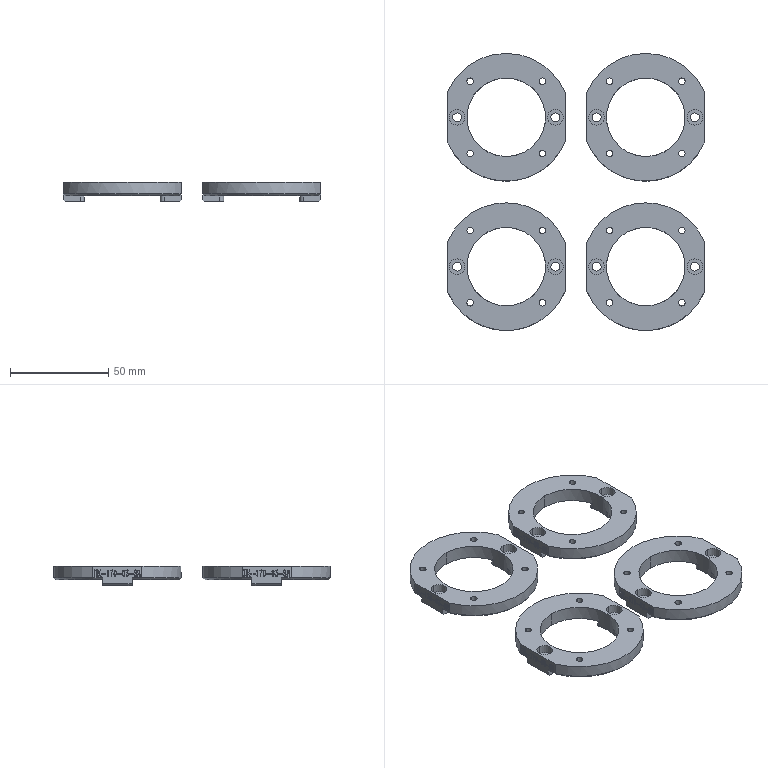NC program | NX | posted with a generic post | part box 131 x 141 x 10 mm
Whole program:
N10 G17 G21 G94 G90
(HOLE_MILLING_1 , TOOL : D6)
N12 T12 M6
N14 G54
N16 G17 G0 G90 X0. Y25. S9500 M3
N18 G43 Z30. H12
N20 Z0.5
N22 G94 G3 X0.5 Y25.5 R0.5 F1450.
N24 X0. Y26. R0.5
N26 X0. Y26. Z0. I0. J-1.
N28 X0. Y26. Z-0.5 I0. J-1.
N30 X0. Y26. Z-1. I0. J-1.
N32 X0. Y26. Z-1.5 I0. J-1.
N34 X0. Y26. Z-2. I0. J-1.
N36 X0. Y26. Z-2.5 I0. J-1.
N38 X0. Y26. Z-3. I0. J-1.
N40 X0. Y26. Z-3.5 I0. J-1.
N42 X0. Y26. Z-4. I0. J-1.
N44 X0.951 Y25.309 Z-4.4 R-1.
N46 X-0.309 Y25.951 R1.
N48 X0.951 Y25.309 R-1.
N50 X0.321 Y25.63 R0.5
N52 X0. Y25. R0.5
N54 G0 Z30.
N56 Y-25.
N58 Z0.5
N60 G3 X0.5 Y-24.5 R0.5
N62 X0. Y-24. R0.5
N64 X0. Y-24. Z0. I0. J-1.
N66 X0. Y-24. Z-0.5 I0. J-1.
N68 X0. Y-24. Z-1. I0. J-1.
N70 X0. Y-24. Z-1.5 I0. J-1.
N72 X0. Y-24. Z-2. I0. J-1.
N74 X0. Y-24. Z-2.5 I0. J-1.
N76 X0. Y-24. Z-3. I0. J-1.
N78 X0. Y-24. Z-3.5 I0. J-1.
N80 X0. Y-24. Z-4. I0. J-1.
N82 X0.951 Y-24.691 Z-4.4 R-1.
N84 X-0.309 Y-24.049 R1.
N86 X0.951 Y-24.691 R-1.
N88 X0.321 Y-24.37 R0.5
N90 X0. Y-25. R0.5
N92 G0 Z30.
N94 M5
(PLANAR_MILL_COPY_COPY_COPY_COPY_COPY_1 , TOOL : D6A45)
N96 T01 M6
N98 G54
N100 G17 G0 G90 X18.452 Y18.385 S9500 M3
N102 G43 Z30. H1
N104 Z0.
N106 G94 G1 Z-1.5 F1250.
N108 G3 X18.385 Y18.635 R0.5
N110 X18.135 Y18.385 R0.25
N112 X18.385 Y18.635 R-0.25
N114 X18.318 Y18.385 R0.5
N116 G1 Z0.
N118 G0 Z30.
N120 X0.866 Y27.1
N122 Z0.
N124 G1 Z-1.5
N126 G3 X0. Y27.6 R1.
N128 X-2.6 Y25. R2.6
N130 X0. Y27.6 R-2.6
N132 X-0.866 Y27.1 R1.
N134 G1 Z0.
N136 G0 Z30.
N138 X-18.318 Y18.385
N140 Z0.
N142 G1 Z-1.5
N144 G3 X-18.385 Y18.635 R0.5
N146 X-18.635 Y18.385 R0.25
N148 X-18.385 Y18.635 R-0.25
N150 X-18.452 Y18.385 R0.5
N152 G1 Z0.
N154 G0 Z30.
N156 X-0.866 Y31.9
N158 Z0.
N160 G1 Z-1.5
N162 G3 X0. Y31.4 R1.
N164 G1 X12.5
N166 G2 X13.038 Y31.292 R1.4
N168 X13.038 Y-31.292 R33.9
N170 X12.5 Y-31.4 R1.4
N172 G1 X-12.5
N174 G2 X-13.038 Y-31.292 R1.4
N176 X-13.038 Y31.292 R33.9
N178 X-12.5 Y31.4 R1.4
N180 G1 X0.
N182 G3 X0.866 Y31.9 R1.
N184 G1 Z0.
N186 G0 Z30.
N188 Y18.1
N190 Z0.
N192 G1 Z-1.5
N194 G3 X0. Y18.6 R1.
N196 X-18.6 Y0. R18.6
N198 X0. Y18.6 R-18.6
N200 X-0.866 Y18.1 R1.
N202 G1 Z0.
N204 G0 Z30.
N206 X18.318 Y-18.385
N208 Z0.
N210 G1 Z-1.5
N212 G3 X18.385 Y-18.635 R0.5
N214 X18.635 Y-18.385 R0.25
N216 X18.385 Y-18.635 R-0.25
N218 X18.452 Y-18.385 R0.5
N220 G1 Z0.
N222 G0 Z30.
N224 X-0.866 Y-27.1
N226 Z0.
N228 G1 Z-1.5
N230 G3 X0. Y-27.6 R1.
N232 X2.6 Y-25. R2.6
N234 X0. Y-27.6 R-2.6
N236 X0.866 Y-27.1 R1.
N238 G1 Z0.
N240 G0 Z30.
N242 X-18.452 Y-18.385
N244 Z0.
N246 G1 Z-1.5
N248 G3 X-18.385 Y-18.635 R0.5
N250 X-18.135 Y-18.385 R0.25
N252 X-18.385 Y-18.635 R-0.25
N254 X-18.318 Y-18.385 R0.5
N256 G1 Z0.
N258 G0 Z30.
N260 M5
N262 M2